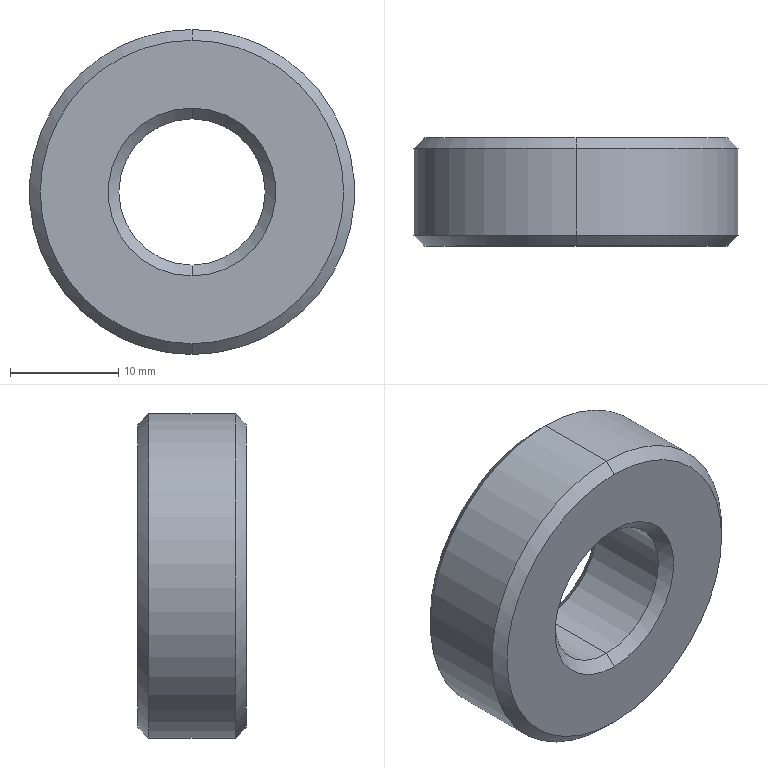Part | Creo | 1 solid | 14 faces | box 30 x 10 x 30 mm | volume 5501 mm3 | cone 8 | cylinder 4 | plane 2 | commonest cylinder face diameters 13.5 x2 30 x2
STEP:
#1=CARTESIAN_POINT('',(0.2584,535.92,-28.25));
#2=VERTEX_POINT('',#1);
#3=CARTESIAN_POINT('',(0.2584,535.92,-41.75));
#4=VERTEX_POINT('',#3);
#5=CARTESIAN_POINT('',(0.2584,535.92,-35.));
#6=DIRECTION('',(0.,1.,0.));
#7=DIRECTION('',(0.,0.,1.));
#8=AXIS2_PLACEMENT_3D('',#5,#6,#7);
#9=CIRCLE('',#8,6.75);
#10=EDGE_CURVE('',#2,#4,#9,.T.);
#11=ORIENTED_EDGE('',*,*,#10,.T.);
#12=CARTESIAN_POINT('',(0.2584,543.92,-41.75));
#13=VERTEX_POINT('',#12);
#14=CARTESIAN_POINT('',(0.2584,543.92,-41.75));
#15=DIRECTION('',(0.,-1.,0.));
#16=VECTOR('',#15,8.);
#17=LINE('',#14,#16);
#18=EDGE_CURVE('',#13,#4,#17,.T.);
#19=ORIENTED_EDGE('',*,*,#18,.F.);
#20=CARTESIAN_POINT('',(0.2584,543.92,-28.25));
#21=VERTEX_POINT('',#20);
#22=CARTESIAN_POINT('',(0.2584,543.92,-35.));
#23=DIRECTION('',(0.,-1.,0.));
#24=DIRECTION('',(0.,0.,-1.));
#25=AXIS2_PLACEMENT_3D('',#22,#23,#24);
#26=CIRCLE('',#25,6.75);
#27=EDGE_CURVE('',#13,#21,#26,.T.);
#28=ORIENTED_EDGE('',*,*,#27,.T.);
#29=CARTESIAN_POINT('',(0.2584,543.92,-28.25));
#30=DIRECTION('',(0.,-1.,0.));
#31=VECTOR('',#30,8.);
#32=LINE('',#29,#31);
#33=EDGE_CURVE('',#21,#2,#32,.T.);
#34=ORIENTED_EDGE('',*,*,#33,.T.);
#35=EDGE_LOOP('',(#11,#19,#28,#34));
#36=FACE_OUTER_BOUND('',#35,.F.);
#37=CARTESIAN_POINT('',(0.2584,544.92,-35.));
#38=DIRECTION('',(0.,-1.,0.));
#39=DIRECTION('',(0.,0.,-1.));
#40=AXIS2_PLACEMENT_3D('',#37,#38,#39);
#41=CYLINDRICAL_SURFACE('',#40,6.75);
#42=ADVANCED_FACE('',(#36),#41,.F.);
#43=ORIENTED_EDGE('',*,*,#10,.F.);
#44=CARTESIAN_POINT('',(0.2584,534.92,-27.25));
#45=VERTEX_POINT('',#44);
#46=CARTESIAN_POINT('',(0.2584,535.92,-28.25));
#47=DIRECTION('',(0.,-0.7071,0.7071));
#48=VECTOR('',#47,1.414);
#49=LINE('',#46,#48);
#50=EDGE_CURVE('',#2,#45,#49,.T.);
#51=ORIENTED_EDGE('',*,*,#50,.T.);
#52=CARTESIAN_POINT('',(0.2584,534.92,-42.75));
#53=VERTEX_POINT('',#52);
#54=CARTESIAN_POINT('',(0.2584,534.92,-35.));
#55=DIRECTION('',(0.,1.,0.));
#56=DIRECTION('',(0.,0.,1.));
#57=AXIS2_PLACEMENT_3D('',#54,#55,#56);
#58=CIRCLE('',#57,7.75);
#59=EDGE_CURVE('',#45,#53,#58,.T.);
#60=ORIENTED_EDGE('',*,*,#59,.T.);
#61=CARTESIAN_POINT('',(0.2584,535.92,-41.75));
#62=DIRECTION('',(0.,-0.7071,-0.7071));
#63=VECTOR('',#62,1.414);
#64=LINE('',#61,#63);
#65=EDGE_CURVE('',#4,#53,#64,.T.);
#66=ORIENTED_EDGE('',*,*,#65,.F.);
#67=EDGE_LOOP('',(#43,#51,#60,#66));
#68=FACE_OUTER_BOUND('',#67,.F.);
#69=CARTESIAN_POINT('',(0.2584,535.42,-35.));
#70=DIRECTION('',(0.,-1.,0.));
#71=DIRECTION('',(0.,0.,1.));
#72=AXIS2_PLACEMENT_3D('',#69,#70,#71);
#73=CONICAL_SURFACE('',#72,7.25,45.);
#74=ADVANCED_FACE('',(#68),#73,.F.);
#75=CARTESIAN_POINT('',(0.2584,535.92,-35.));
#76=DIRECTION('',(0.,1.,0.));
#77=DIRECTION('',(0.,0.,-1.));
#78=AXIS2_PLACEMENT_3D('',#75,#76,#77);
#79=CIRCLE('',#78,6.75);
#80=EDGE_CURVE('',#4,#2,#79,.T.);
#81=ORIENTED_EDGE('',*,*,#80,.F.);
#82=ORIENTED_EDGE('',*,*,#65,.T.);
#83=CARTESIAN_POINT('',(0.2584,534.92,-35.));
#84=DIRECTION('',(0.,1.,0.));
#85=DIRECTION('',(0.,0.,-1.));
#86=AXIS2_PLACEMENT_3D('',#83,#84,#85);
#87=CIRCLE('',#86,7.75);
#88=EDGE_CURVE('',#53,#45,#87,.T.);
#89=ORIENTED_EDGE('',*,*,#88,.T.);
#90=ORIENTED_EDGE('',*,*,#50,.F.);
#91=EDGE_LOOP('',(#81,#82,#89,#90));
#92=FACE_OUTER_BOUND('',#91,.F.);
#93=CARTESIAN_POINT('',(0.2584,535.42,-35.));
#94=DIRECTION('',(0.,-1.,0.));
#95=DIRECTION('',(0.,0.,1.));
#96=AXIS2_PLACEMENT_3D('',#93,#94,#95);
#97=CONICAL_SURFACE('',#96,7.25,45.);
#98=ADVANCED_FACE('',(#92),#97,.F.);
#99=ORIENTED_EDGE('',*,*,#80,.T.);
#100=ORIENTED_EDGE('',*,*,#33,.F.);
#101=CARTESIAN_POINT('',(0.2584,543.92,-35.));
#102=DIRECTION('',(0.,-1.,0.));
#103=DIRECTION('',(0.,0.,1.));
#104=AXIS2_PLACEMENT_3D('',#101,#102,#103);
#105=CIRCLE('',#104,6.75);
#106=EDGE_CURVE('',#21,#13,#105,.T.);
#107=ORIENTED_EDGE('',*,*,#106,.T.);
#108=ORIENTED_EDGE('',*,*,#18,.T.);
#109=EDGE_LOOP('',(#99,#100,#107,#108));
#110=FACE_OUTER_BOUND('',#109,.F.);
#111=CARTESIAN_POINT('',(0.2584,544.92,-35.));
#112=DIRECTION('',(0.,-1.,0.));
#113=DIRECTION('',(0.,0.,-1.));
#114=AXIS2_PLACEMENT_3D('',#111,#112,#113);
#115=CYLINDRICAL_SURFACE('',#114,6.75);
#116=ADVANCED_FACE('',(#110),#115,.F.);
#117=CARTESIAN_POINT('',(0.2584,544.92,-27.25));
#118=VERTEX_POINT('',#117);
#119=CARTESIAN_POINT('',(0.2584,544.92,-42.75));
#120=VERTEX_POINT('',#119);
#121=CARTESIAN_POINT('',(0.2584,544.92,-35.));
#122=DIRECTION('',(0.,-1.,0.));
#123=DIRECTION('',(0.,0.,1.));
#124=AXIS2_PLACEMENT_3D('',#121,#122,#123);
#125=CIRCLE('',#124,7.75);
#126=EDGE_CURVE('',#118,#120,#125,.T.);
#127=ORIENTED_EDGE('',*,*,#126,.T.);
#128=CARTESIAN_POINT('',(0.2584,543.92,-41.75));
#129=DIRECTION('',(0.,0.7071,-0.7071));
#130=VECTOR('',#129,1.414);
#131=LINE('',#128,#130);
#132=EDGE_CURVE('',#13,#120,#131,.T.);
#133=ORIENTED_EDGE('',*,*,#132,.F.);
#134=ORIENTED_EDGE('',*,*,#106,.F.);
#135=CARTESIAN_POINT('',(0.2584,543.92,-28.25));
#136=DIRECTION('',(0.,0.7071,0.7071));
#137=VECTOR('',#136,1.414);
#138=LINE('',#135,#137);
#139=EDGE_CURVE('',#21,#118,#138,.T.);
#140=ORIENTED_EDGE('',*,*,#139,.T.);
#141=EDGE_LOOP('',(#127,#133,#134,#140));
#142=FACE_OUTER_BOUND('',#141,.F.);
#143=CARTESIAN_POINT('',(0.2584,544.42,-35.));
#144=DIRECTION('',(0.,1.,0.));
#145=DIRECTION('',(0.,0.,-1.));
#146=AXIS2_PLACEMENT_3D('',#143,#144,#145);
#147=CONICAL_SURFACE('',#146,7.25,45.);
#148=ADVANCED_FACE('',(#142),#147,.F.);
#149=CARTESIAN_POINT('',(0.2584,544.92,-49.));
#150=VERTEX_POINT('',#149);
#151=CARTESIAN_POINT('',(0.2584,544.92,-21.));
#152=VERTEX_POINT('',#151);
#153=CARTESIAN_POINT('',(0.2584,544.92,-35.));
#154=DIRECTION('',(0.,1.,0.));
#155=DIRECTION('',(0.,0.,-1.));
#156=AXIS2_PLACEMENT_3D('',#153,#154,#155);
#157=CIRCLE('',#156,14.);
#158=EDGE_CURVE('',#150,#152,#157,.T.);
#159=ORIENTED_EDGE('',*,*,#158,.F.);
#160=CARTESIAN_POINT('',(0.2584,544.92,-35.));
#161=DIRECTION('',(0.,1.,0.));
#162=DIRECTION('',(0.,0.,1.));
#163=AXIS2_PLACEMENT_3D('',#160,#161,#162);
#164=CIRCLE('',#163,14.);
#165=EDGE_CURVE('',#152,#150,#164,.T.);
#166=ORIENTED_EDGE('',*,*,#165,.F.);
#167=EDGE_LOOP('',(#159,#166));
#168=FACE_OUTER_BOUND('',#167,.F.);
#169=CARTESIAN_POINT('',(0.2584,544.92,-35.));
#170=DIRECTION('',(0.,-1.,0.));
#171=DIRECTION('',(0.,0.,-1.));
#172=AXIS2_PLACEMENT_3D('',#169,#170,#171);
#173=CIRCLE('',#172,7.75);
#174=EDGE_CURVE('',#120,#118,#173,.T.);
#175=ORIENTED_EDGE('',*,*,#174,.F.);
#176=ORIENTED_EDGE('',*,*,#126,.F.);
#177=EDGE_LOOP('',(#175,#176));
#178=FACE_BOUND('',#177,.F.);
#179=CARTESIAN_POINT('',(0.2584,544.92,-35.));
#180=DIRECTION('',(0.,-1.,0.));
#181=DIRECTION('',(0.,0.,-1.));
#182=AXIS2_PLACEMENT_3D('',#179,#180,#181);
#183=PLANE('',#182);
#184=ADVANCED_FACE('',(#168,#178),#183,.F.);
#185=ORIENTED_EDGE('',*,*,#174,.T.);
#186=ORIENTED_EDGE('',*,*,#139,.F.);
#187=ORIENTED_EDGE('',*,*,#27,.F.);
#188=ORIENTED_EDGE('',*,*,#132,.T.);
#189=EDGE_LOOP('',(#185,#186,#187,#188));
#190=FACE_OUTER_BOUND('',#189,.F.);
#191=CARTESIAN_POINT('',(0.2584,544.42,-35.));
#192=DIRECTION('',(0.,1.,0.));
#193=DIRECTION('',(0.,0.,-1.));
#194=AXIS2_PLACEMENT_3D('',#191,#192,#193);
#195=CONICAL_SURFACE('',#194,7.25,45.);
#196=ADVANCED_FACE('',(#190),#195,.F.);
#197=ORIENTED_EDGE('',*,*,#158,.T.);
#198=CARTESIAN_POINT('',(0.2584,543.92,-20.));
#199=VERTEX_POINT('',#198);
#200=CARTESIAN_POINT('',(0.2584,544.92,-21.));
#201=DIRECTION('',(0.,-0.7071,0.7071));
#202=VECTOR('',#201,1.414);
#203=LINE('',#200,#202);
#204=EDGE_CURVE('',#152,#199,#203,.T.);
#205=ORIENTED_EDGE('',*,*,#204,.T.);
#206=CARTESIAN_POINT('',(0.2584,543.92,-50.));
#207=VERTEX_POINT('',#206);
#208=CARTESIAN_POINT('',(0.2584,543.92,-35.));
#209=DIRECTION('',(0.,1.,0.));
#210=DIRECTION('',(0.,0.,-1.));
#211=AXIS2_PLACEMENT_3D('',#208,#209,#210);
#212=CIRCLE('',#211,15.);
#213=EDGE_CURVE('',#207,#199,#212,.T.);
#214=ORIENTED_EDGE('',*,*,#213,.F.);
#215=CARTESIAN_POINT('',(0.2584,544.92,-49.));
#216=DIRECTION('',(0.,-0.7071,-0.7071));
#217=VECTOR('',#216,1.414);
#218=LINE('',#215,#217);
#219=EDGE_CURVE('',#150,#207,#218,.T.);
#220=ORIENTED_EDGE('',*,*,#219,.F.);
#221=EDGE_LOOP('',(#197,#205,#214,#220));
#222=FACE_OUTER_BOUND('',#221,.F.);
#223=CARTESIAN_POINT('',(0.2584,544.42,-35.));
#224=DIRECTION('',(0.,-1.,0.));
#225=DIRECTION('',(0.,0.,1.));
#226=AXIS2_PLACEMENT_3D('',#223,#224,#225);
#227=CONICAL_SURFACE('',#226,14.5,45.);
#228=ADVANCED_FACE('',(#222),#227,.T.);
#229=ORIENTED_EDGE('',*,*,#165,.T.);
#230=ORIENTED_EDGE('',*,*,#219,.T.);
#231=CARTESIAN_POINT('',(0.2584,543.92,-35.));
#232=DIRECTION('',(0.,1.,0.));
#233=DIRECTION('',(0.,0.,1.));
#234=AXIS2_PLACEMENT_3D('',#231,#232,#233);
#235=CIRCLE('',#234,15.);
#236=EDGE_CURVE('',#199,#207,#235,.T.);
#237=ORIENTED_EDGE('',*,*,#236,.F.);
#238=ORIENTED_EDGE('',*,*,#204,.F.);
#239=EDGE_LOOP('',(#229,#230,#237,#238));
#240=FACE_OUTER_BOUND('',#239,.F.);
#241=CARTESIAN_POINT('',(0.2584,544.42,-35.));
#242=DIRECTION('',(0.,-1.,0.));
#243=DIRECTION('',(0.,0.,1.));
#244=AXIS2_PLACEMENT_3D('',#241,#242,#243);
#245=CONICAL_SURFACE('',#244,14.5,45.);
#246=ADVANCED_FACE('',(#240),#245,.T.);
#247=CARTESIAN_POINT('',(0.2584,535.92,-50.));
#248=VERTEX_POINT('',#247);
#249=CARTESIAN_POINT('',(0.2584,535.92,-20.));
#250=VERTEX_POINT('',#249);
#251=CARTESIAN_POINT('',(0.2584,535.92,-35.));
#252=DIRECTION('',(0.,-1.,0.));
#253=DIRECTION('',(0.,0.,-1.));
#254=AXIS2_PLACEMENT_3D('',#251,#252,#253);
#255=CIRCLE('',#254,15.);
#256=EDGE_CURVE('',#248,#250,#255,.T.);
#257=ORIENTED_EDGE('',*,*,#256,.T.);
#258=CARTESIAN_POINT('',(0.2584,543.92,-20.));
#259=DIRECTION('',(0.,-1.,0.));
#260=VECTOR('',#259,8.);
#261=LINE('',#258,#260);
#262=EDGE_CURVE('',#199,#250,#261,.T.);
#263=ORIENTED_EDGE('',*,*,#262,.F.);
#264=ORIENTED_EDGE('',*,*,#236,.T.);
#265=CARTESIAN_POINT('',(0.2584,543.92,-50.));
#266=DIRECTION('',(0.,-1.,0.));
#267=VECTOR('',#266,8.);
#268=LINE('',#265,#267);
#269=EDGE_CURVE('',#207,#248,#268,.T.);
#270=ORIENTED_EDGE('',*,*,#269,.T.);
#271=EDGE_LOOP('',(#257,#263,#264,#270));
#272=FACE_OUTER_BOUND('',#271,.F.);
#273=CARTESIAN_POINT('',(0.2584,544.92,-35.));
#274=DIRECTION('',(0.,-1.,0.));
#275=DIRECTION('',(0.,0.,-1.));
#276=AXIS2_PLACEMENT_3D('',#273,#274,#275);
#277=CYLINDRICAL_SURFACE('',#276,15.);
#278=ADVANCED_FACE('',(#272),#277,.T.);
#279=ORIENTED_EDGE('',*,*,#256,.F.);
#280=CARTESIAN_POINT('',(0.2584,534.92,-49.));
#281=VERTEX_POINT('',#280);
#282=CARTESIAN_POINT('',(0.2584,534.92,-49.));
#283=DIRECTION('',(0.,0.7071,-0.7071));
#284=VECTOR('',#283,1.414);
#285=LINE('',#282,#284);
#286=EDGE_CURVE('',#281,#248,#285,.T.);
#287=ORIENTED_EDGE('',*,*,#286,.F.);
#288=CARTESIAN_POINT('',(0.2584,534.92,-21.));
#289=VERTEX_POINT('',#288);
#290=CARTESIAN_POINT('',(0.2584,534.92,-35.));
#291=DIRECTION('',(0.,-1.,0.));
#292=DIRECTION('',(0.,0.,-1.));
#293=AXIS2_PLACEMENT_3D('',#290,#291,#292);
#294=CIRCLE('',#293,14.);
#295=EDGE_CURVE('',#281,#289,#294,.T.);
#296=ORIENTED_EDGE('',*,*,#295,.T.);
#297=CARTESIAN_POINT('',(0.2584,534.92,-21.));
#298=DIRECTION('',(0.,0.7071,0.7071));
#299=VECTOR('',#298,1.414);
#300=LINE('',#297,#299);
#301=EDGE_CURVE('',#289,#250,#300,.T.);
#302=ORIENTED_EDGE('',*,*,#301,.T.);
#303=EDGE_LOOP('',(#279,#287,#296,#302));
#304=FACE_OUTER_BOUND('',#303,.F.);
#305=CARTESIAN_POINT('',(0.2584,535.42,-35.));
#306=DIRECTION('',(0.,1.,0.));
#307=DIRECTION('',(0.,0.,-1.));
#308=AXIS2_PLACEMENT_3D('',#305,#306,#307);
#309=CONICAL_SURFACE('',#308,14.5,45.);
#310=ADVANCED_FACE('',(#304),#309,.T.);
#311=CARTESIAN_POINT('',(0.2584,535.92,-35.));
#312=DIRECTION('',(0.,-1.,0.));
#313=DIRECTION('',(0.,0.,1.));
#314=AXIS2_PLACEMENT_3D('',#311,#312,#313);
#315=CIRCLE('',#314,15.);
#316=EDGE_CURVE('',#250,#248,#315,.T.);
#317=ORIENTED_EDGE('',*,*,#316,.F.);
#318=ORIENTED_EDGE('',*,*,#301,.F.);
#319=CARTESIAN_POINT('',(0.2584,534.92,-35.));
#320=DIRECTION('',(0.,-1.,0.));
#321=DIRECTION('',(0.,0.,1.));
#322=AXIS2_PLACEMENT_3D('',#319,#320,#321);
#323=CIRCLE('',#322,14.);
#324=EDGE_CURVE('',#289,#281,#323,.T.);
#325=ORIENTED_EDGE('',*,*,#324,.T.);
#326=ORIENTED_EDGE('',*,*,#286,.T.);
#327=EDGE_LOOP('',(#317,#318,#325,#326));
#328=FACE_OUTER_BOUND('',#327,.F.);
#329=CARTESIAN_POINT('',(0.2584,535.42,-35.));
#330=DIRECTION('',(0.,1.,0.));
#331=DIRECTION('',(0.,0.,-1.));
#332=AXIS2_PLACEMENT_3D('',#329,#330,#331);
#333=CONICAL_SURFACE('',#332,14.5,45.);
#334=ADVANCED_FACE('',(#328),#333,.T.);
#335=ORIENTED_EDGE('',*,*,#316,.T.);
#336=ORIENTED_EDGE('',*,*,#269,.F.);
#337=ORIENTED_EDGE('',*,*,#213,.T.);
#338=ORIENTED_EDGE('',*,*,#262,.T.);
#339=EDGE_LOOP('',(#335,#336,#337,#338));
#340=FACE_OUTER_BOUND('',#339,.F.);
#341=CARTESIAN_POINT('',(0.2584,544.92,-35.));
#342=DIRECTION('',(0.,-1.,0.));
#343=DIRECTION('',(0.,0.,-1.));
#344=AXIS2_PLACEMENT_3D('',#341,#342,#343);
#345=CYLINDRICAL_SURFACE('',#344,15.);
#346=ADVANCED_FACE('',(#340),#345,.T.);
#347=ORIENTED_EDGE('',*,*,#295,.F.);
#348=ORIENTED_EDGE('',*,*,#324,.F.);
#349=EDGE_LOOP('',(#347,#348));
#350=FACE_OUTER_BOUND('',#349,.F.);
#351=ORIENTED_EDGE('',*,*,#88,.F.);
#352=ORIENTED_EDGE('',*,*,#59,.F.);
#353=EDGE_LOOP('',(#351,#352));
#354=FACE_BOUND('',#353,.F.);
#355=CARTESIAN_POINT('',(0.2584,534.92,-35.));
#356=DIRECTION('',(0.,-1.,0.));
#357=DIRECTION('',(0.,0.,-1.));
#358=AXIS2_PLACEMENT_3D('',#355,#356,#357);
#359=PLANE('',#358);
#360=ADVANCED_FACE('',(#350,#354),#359,.T.);
#361=CLOSED_SHELL('',(#42,#74,#98,#116,#148,#184,#196,#228,#246,#278,#310,#334,#346,#360));
#362=MANIFOLD_SOLID_BREP('',#361);
#363=(LENGTH_UNIT()NAMED_UNIT(*)SI_UNIT(.MILLI.,.METRE.));
#364=UNCERTAINTY_MEASURE_WITH_UNIT(LENGTH_MEASURE(0.004359),#363,'','');
#365=(NAMED_UNIT(*)PLANE_ANGLE_UNIT()SI_UNIT($,.RADIAN.));
#366=PLANE_ANGLE_MEASURE_WITH_UNIT(PLANE_ANGLE_MEASURE(0.01745),#365);
#367=(CONVERSION_BASED_UNIT('DEGREE',#366)NAMED_UNIT(*)PLANE_ANGLE_UNIT());
#368=(NAMED_UNIT(*)SI_UNIT($,.STERADIAN.)SOLID_ANGLE_UNIT());
#369=(GEOMETRIC_REPRESENTATION_CONTEXT(3)GLOBAL_UNCERTAINTY_ASSIGNED_CONTEXT((#364))GLOBAL_UNIT_ASSIGNED_CONTEXT((#363,#367,#368))REPRESENTATION_CONTEXT('',''));
#370=ADVANCED_BREP_SHAPE_REPRESENTATION('',(#362),#369);